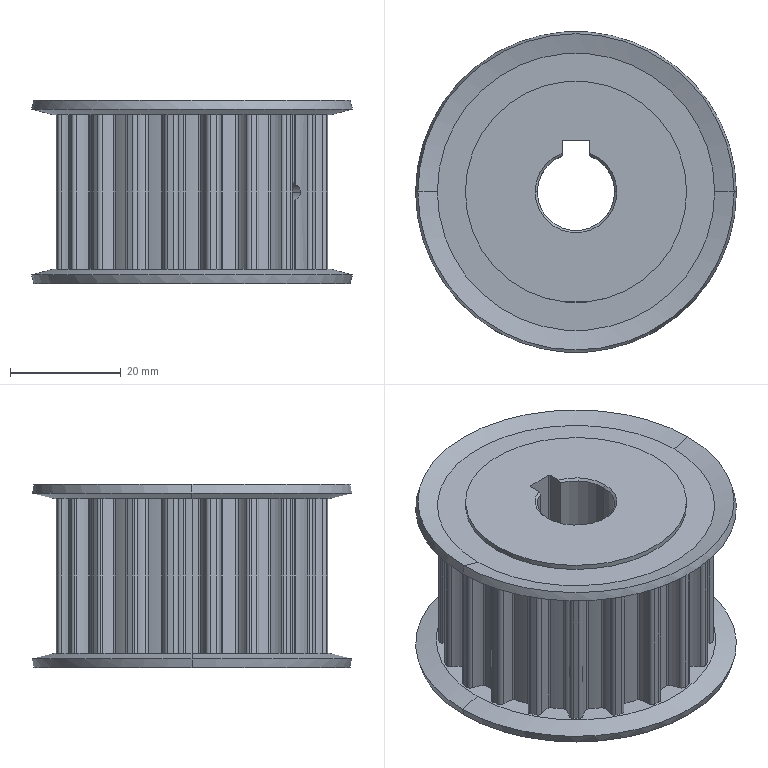Part | SolidWorks | features MBimport 1 | 1 solid | 228 faces | box 58 x 58 x 33.085 mm | volume 51729 mm3 | cylinder 201 | cone 18 | plane 9 | commonest cylinder face diameters 0.8 x51 1.5 x50 10.6 x44 43.9 x23 49.56 x20 4.134 x4